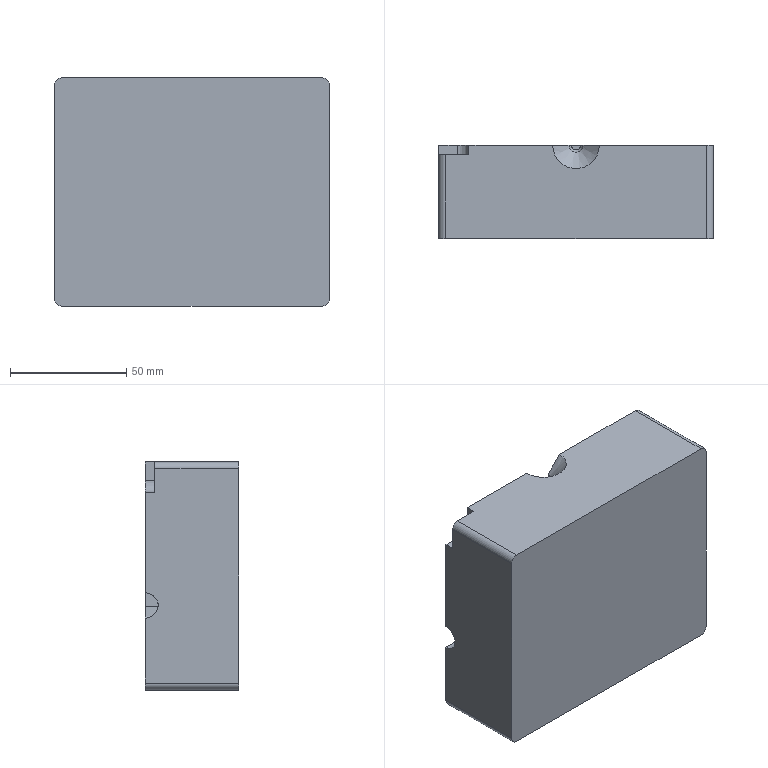NC program | NX | posted with a generic post | part box 118 x 40 x 98 mm
Lines 2681 to 3706 of 39656:
(CONTOUR_AREA , TOOL : B4)
N5348 M6
N5350 G54
N5352 G17 G0 G90 X34.942 Y6.616 S0 M3
N5354 G43 Z30. H0
N5356 Z1.2
N5358 G94 G1 Z-2.023 F250.
N5360 G2 X36.94 Y4.614 R2.
N5362 G1 Y4.41 Z-2.031
N5364 X36.938 Y4.351 Z-2.037
N5366 X36.937 Y4.333 Z-2.04
N5368 X36.906 Y4.326 Z-2.039
N5370 X36.749 Y4.28 Z-2.021
N5372 X36.703 Y4.272 Z-2.019
N5374 X36.7 Y4.271
N5376 X36.569 Y4.211 Z-2.015
N5378 X36.556 Y4.205 Z-2.014
N5380 X36.424 Y4.139 Z-2.012
N5382 X36.353 Y4.099 Z-2.011
N5384 X36.299 Y4.065 Z-2.01
N5386 X36.22 Y4.012 Z-2.009
N5388 X36.181 Y3.984
N5390 X36.069 Y3.896 Z-2.01
N5392 X35.957 Y3.79 Z-2.012
N5394 X35.871 Y3.697 Z-2.009
N5396 X35.8 Y3.611 Z-2.006
N5398 X35.781 Y3.588
N5400 X35.69 Y3.455 Z-2.004
N5402 X35.625 Y3.346 Z-2.003
N5404 X35.558 Y3.211 Z-2.002
N5406 X35.5 Y3.072 Z-2.003
N5408 X35.479 Y3.012 Z-2.004
N5410 X35.451 Y2.921
N5412 X35.435 Y2.861 Z-2.005
N5414 X35.43 Y2.837
N5416 X35.429 Y2.833 Z-1.999
N5418 X35.43 Y2.836 Z-2.004
N5420 X35.422 Y2.802 Z-2.005
N5422 X35.413 Y2.76
N5424 X35.39 Y2.612 Z-2.006
N5426 X35.377 Y2.412 Z-2.007
N5428 Y2.288
N5430 Y1.813 Z-2.009
N5432 Y-1.384 Z-2.01
N5434 Y-2.583 Z-2.008
N5436 Y-3.382 Z-1.999
N5438 Y-3.482 Z-1.998
N5440 Y-3.582 Z-2.
N5442 Y-3.61 Z-2.004
N5444 Y-3.611 Z-2.006
N5446 X35.376 Y-3.613 Z-2.02
N5448 X35.361 Z-2.375
N5450 X35.312 Z-2.767
N5452 X35.304 Z-2.804
N5454 X35.262 Z-3.01
N5456 X35.163 Z-3.365
N5458 X35.095 Z-3.558
N5460 X35.064 Z-3.647
N5462 X35.033 Z-3.717
N5464 X34.965 Z-3.877
N5466 X34.767 Z-4.256
N5468 X34.568 Z-4.565
N5470 X34.37 Z-4.83
N5472 X34.172 Z-5.055
N5474 X33.973 Z-5.255
N5476 X33.775 Z-5.431
N5478 X33.577 Z-5.588
N5480 X33.379 Z-5.728
N5482 X33.18 Z-5.853
N5484 X32.982 Z-5.962
N5486 X32.784 Z-6.062
N5488 X32.585 Z-6.148
N5490 X32.387 Z-6.223
N5492 X32.189 Z-6.287
N5494 X31.991 Z-6.342
N5496 X31.792 Z-6.388
N5498 X31.594 Z-6.423
N5500 X31.396 Z-6.449
N5502 X31.197 Z-6.467
N5504 X30.999 Z-6.475
N5506 X30.801
N5508 X30.603 Z-6.467
N5510 X30.404 Z-6.449
N5512 X30.206 Z-6.423
N5514 X30.008 Z-6.388
N5516 X29.809 Z-6.342
N5518 X29.611 Z-6.287
N5520 X29.413 Z-6.223
N5522 X29.215 Z-6.148
N5524 X29.016 Z-6.061
N5526 X28.818 Z-5.964
N5528 X28.62 Z-5.853
N5530 X28.421 Z-5.728
N5532 X28.223 Z-5.588
N5534 X28.025 Z-5.431
N5536 X27.827 Z-5.255
N5538 X27.628 Z-5.056
N5540 X27.43 Z-4.83
N5542 X27.232 Z-4.565
N5544 X27.033 Z-4.255
N5546 X26.835 Z-3.875
N5548 X26.82 Z-3.842
N5550 X26.736 Z-3.647
N5552 X26.705 Z-3.558
N5554 X26.629 Z-3.343
N5556 X26.587 Z-3.203
N5558 X26.58 Z-3.174
N5560 X26.538 Z-3.01
N5562 X26.533 Z-2.985
N5564 X26.488 Z-2.767
N5566 X26.439 Z-2.375
N5568 X26.437 Y-3.611 Z-2.364
N5570 X26.428 Y-3.582 Z-2.191
N5572 X26.426 Y-3.517 Z-2.156
N5574 Y-3.478 Z-2.137
N5576 X26.425 Y-3.382 Z-2.107
N5578 Y-3.275 Z-2.077
N5580 X26.424 Y-3.182 Z-2.062
N5582 Y-3.02 Z-2.037
N5584 Y-2.983 Z-2.034
N5586 X26.423 Y-2.798 Z-2.021
N5588 Y-2.589 Z-2.014
N5590 Y-2.184 Z-2.01
N5592 Y0.614
N5594 Y2.212 Z-2.007
N5596 Y2.412
N5598 X26.41 Y2.612 Z-2.006
N5600 X26.387 Y2.76 Z-2.005
N5602 X26.376 Y2.812
N5604 X26.365 Y2.861
N5606 X26.349 Y2.921 Z-2.004
N5608 X26.321 Y3.011
N5610 X26.3 Y3.072 Z-2.003
N5612 X26.24 Y3.216
N5614 X26.175 Y3.346 Z-2.005
N5616 X26.101 Y3.471 Z-2.007
N5618 X26.044 Y3.552 Z-2.008
N5620 X26.019 Y3.588 Z-2.009
N5622 X26.001 Y3.61
N5624 X25.929 Y3.697 Z-2.011
N5626 X25.844 Y3.789 Z-2.012
N5628 X25.823 Y3.809 Z-2.013
N5630 X25.731 Y3.897 Z-2.012
N5632 X25.619 Y3.984
N5634 X25.582 Y4.011
N5636 X25.501 Y4.065 Z-2.011
N5638 X25.376 Y4.139 Z-2.01
N5640 X25.237 Y4.208 Z-2.009
N5642 X25.095 Y4.265 Z-2.01
N5644 X25.011 Y4.292 Z-2.008
N5646 X24.894 Y4.326 Z-2.003
N5648 X24.881 Y4.329
N5650 X24.872 Y4.331 Z-2.002
N5652 X24.861 Y4.354
N5654 Y4.394 Z-2.004
N5656 Y5.01 Z-2.007
N5658 Y46.77 Z-2.008
N5660 X24.86 Y48.768 Z-2.005
N5662 X24.861 Y48.968 Z-2.007
N5664 X24.859 Y48.984 Z-2.009
N5666 X24.861 Y48.989 Z-2.096
N5668 X24.868 Y48.999 Z-2.295
N5670 X24.87 Y49. Z-2.364
N5672 X24.872 Z-2.387
N5674 X24.877 Z-2.463
N5676 X24.9 Y48.999 Z-2.698
N5678 X24.906 Z-2.741
N5680 X24.927 Z-2.896
N5682 X24.931 Z-2.92
N5684 X24.952 Z-3.051
N5686 X25.051 Z-3.5
N5688 X25.119 Z-3.741
N5690 X25.15 Z-3.851
N5692 X25.181 Z-3.936
N5694 X25.249 Z-4.128
N5696 X25.447 Z-4.597
N5698 X25.645 Z-4.975
N5700 X25.843 Z-5.302
N5702 X26.042 Z-5.587
N5704 X26.24 Z-5.843
N5706 X26.439 Z-6.07
N5708 X26.636 Z-6.276
N5710 X26.835 Z-6.466
N5712 X27.033 Z-6.639
N5714 X27.232 Z-6.798
N5716 X27.43 Z-6.943
N5718 X27.628 Z-7.076
N5720 X27.827 Z-7.199
N5722 X28.025 Z-7.312
N5724 X28.223 Z-7.414
N5726 X28.421 Z-7.507
N5728 X28.62 Z-7.592
N5730 X28.818 Z-7.669
N5732 X29.016 Z-7.738
N5734 X29.215 Z-7.799
N5736 X29.412 Z-7.852
N5738 X29.611 Z-7.901
N5740 X29.809 Z-7.939
N5742 X30.007 Z-7.973
N5744 X30.205 Z-8.
N5746 X30.404 Z-8.019
N5748 X30.601 Z-8.031
N5750 X30.801 Z-8.038
N5752 X30.999
N5754 X31.197 Z-8.032
N5756 X31.396 Z-8.019
N5758 X31.594 Z-8.
N5760 X31.792 Z-7.973
N5762 X31.99 Z-7.94
N5764 X32.189 Z-7.899
N5766 X32.387 Z-7.853
N5768 X32.585 Z-7.799
N5770 X32.784 Z-7.738
N5772 X32.982 Z-7.669
N5774 X33.18 Z-7.592
N5776 X33.379 Z-7.508
N5778 X33.577 Z-7.414
N5780 X33.775 Z-7.311
N5782 X33.973 Z-7.199
N5784 X34.172 Z-7.076
N5786 X34.37 Z-6.943
N5788 X34.568 Z-6.798
N5790 X34.767 Z-6.64
N5792 X34.964 Z-6.466
N5794 X35.163 Z-6.277
N5796 X35.361 Z-6.07
N5798 X35.56 Z-5.843
N5800 X35.758 Z-5.587
N5802 X35.956 Z-5.303
N5804 X36.154 Z-4.976
N5806 X36.353 Z-4.595
N5808 X36.551 Z-4.128
N5810 X36.567 Z-4.088
N5812 X36.65 Z-3.851
N5814 X36.757 Z-3.473
N5816 X36.799 Z-3.301
N5818 X36.843 Z-3.078
N5820 X36.869 Z-2.919
N5822 X36.873 Z-2.897
N5824 X36.898 Z-2.714
N5826 X36.9 Z-2.698
N5828 X36.921 Y49. Z-2.485
N5830 X36.93 Y48.986 Z-2.363
N5832 X36.935 Y48.971 Z-2.232
N5834 Y48.968 Z-2.219
N5836 X36.936 Y48.941 Z-2.201
N5838 X36.937 Y48.768 Z-2.155
N5840 Y48.679 Z-2.132
N5842 X36.938 Y48.568 Z-2.108
N5844 Y48.432 Z-2.08
N5846 Y48.369 Z-2.07
N5848 X36.939 Y48.202 Z-2.046
N5850 Y48.169 Z-2.043
N5852 Y47.985 Z-2.027
N5854 Y47.776 Z-2.018
N5856 Y47.572 Z-2.013
N5858 Y47.17 Z-2.011
N5860 Y42.374 Z-2.018
N5862 X36.94 Y41.175 Z-2.017
N5864 Y40.182 Z-2.007
N5866 Y39.378 Z-2.002
N5868 Y27.389 Z-2.018
N5870 Y6.811
N5872 Y5.215
N5874 Y4.81 Z-2.019
N5876 Y4.614 Z-2.023
N5878 X36.937 Y4.61 Z-2.123
N5880 Y4.383 Z-2.134
N5882 X36.934 Y4.333 Z-2.141
N5884 X36.913 Y4.327 Z-2.14
N5886 X36.906 Y4.326 Z-2.139
N5888 X36.798 Y4.297 Z-2.127
N5890 X36.749 Y4.281 Z-2.121
N5892 X36.742 Y4.28
N5894 X36.719 Y4.276 Z-2.12
N5896 X36.7 Y4.271 Z-2.119
N5898 X36.645 Y4.246 Z-2.117
N5900 X36.551 Y4.203 Z-2.114
N5902 X36.423 Y4.14 Z-2.112
N5904 X36.353 Y4.1 Z-2.111
N5906 X36.298 Y4.066 Z-2.11
N5908 X36.27 Y4.048
N5910 X36.216 Y4.012 Z-2.109
N5912 X36.189 Y3.992
N5914 X36.062 Y3.892 Z-2.11
N5916 X35.956 Y3.791 Z-2.112
N5918 X35.87 Y3.698 Z-2.109
N5920 X35.798 Y3.611 Z-2.106
N5922 X35.785 Y3.595
N5924 X35.758 Y3.559 Z-2.105
N5926 X35.698 Y3.471 Z-2.104
N5928 X35.661 Y3.411
N5930 X35.624 Y3.347 Z-2.103
N5932 X35.56 Y3.22 Z-2.102
N5934 X35.544 Y3.186
N5936 X35.493 Y3.058 Z-2.103
N5938 X35.476 Y3.012 Z-2.104
N5940 X35.463 Y2.966
N5942 X35.45 Y2.923
N5944 X35.428 Y2.84 Z-2.105
N5946 X35.421 Y2.812
N5948 X35.414 Y2.773
N5950 X35.411 Y2.761
N5952 X35.388 Y2.612 Z-2.106
N5954 X35.375 Y2.414 Z-2.107
N5956 Y0.182 Z-2.109
N5958 Y-1.384 Z-2.11
N5960 Y-2.448 Z-2.108
N5962 Y-3.505 Z-2.099
N5964 Y-3.507 Z-2.101
N5966 Y-3.51 Z-2.103
N5968 X35.374 Y-3.511 Z-2.156
N5970 X35.366 Y-3.513 Z-2.299
N5972 X35.361 Z-2.375
N5974 X35.312 Z-2.761
N5976 X35.262 Z-3.006
N5978 X35.213 Z-3.199
N5980 X35.163 Z-3.365
N5982 X35.064 Z-3.644
N5984 X34.965 Z-3.877
N5986 X34.767 Z-4.256
N5988 X34.568 Z-4.565
N5990 X34.37 Z-4.83
N5992 X34.172 Z-5.055
N5994 X33.973 Z-5.255
N5996 X33.775 Z-5.431
N5998 X33.577 Z-5.588
N6000 X33.379 Z-5.728
N6002 X33.18 Z-5.853
N6004 X32.982 Z-5.962
N6006 X32.784 Z-6.062
N6008 X32.585 Z-6.148
N6010 X32.387 Z-6.223
N6012 X32.189 Z-6.287
N6014 X31.991 Z-6.342
N6016 X31.792 Z-6.388
N6018 X31.594 Z-6.423
N6020 X31.396 Z-6.449
N6022 X31.197 Z-6.467
N6024 X30.999 Z-6.475
N6026 X30.801
N6028 X30.603 Z-6.467
N6030 X30.404 Z-6.449
N6032 X30.206 Z-6.423
N6034 X30.008 Z-6.388
N6036 X29.809 Z-6.342
N6038 X29.611 Z-6.287
N6040 X29.413 Z-6.223
N6042 X29.215 Z-6.148
N6044 X29.016 Z-6.061
N6046 X28.818 Z-5.964
N6048 X28.62 Z-5.853
N6050 X28.421 Z-5.728
N6052 X28.223 Z-5.588
N6054 X28.025 Z-5.431
N6056 X27.827 Z-5.255
N6058 X27.628 Z-5.056
N6060 X27.43 Z-4.83
N6062 X27.232 Z-4.565
N6064 X27.033 Z-4.255
N6066 X26.835 Z-3.875
N6068 X26.736 Z-3.644
N6070 X26.637 Z-3.365
N6072 X26.587 Z-3.199
N6074 X26.538 Z-3.006
N6076 X26.505 Z-2.846
N6078 X26.488 Z-2.761
N6080 X26.456 Y-3.511 Z-2.512
N6082 X26.439 Y-3.502 Z-2.375
N6084 X26.433 Y-3.488 Z-2.277
N6086 X26.432 Y-3.484 Z-2.263
N6088 X26.43 Y-3.382 Z-2.215
N6090 X26.429 Y-3.342 Z-2.2
N6092 X26.426 Y-3.182 Z-2.16
N6094 Y-3.161 Z-2.156
N6096 Y-2.949 Z-2.131
N6098 Y-2.787 Z-2.12
N6100 X26.425 Y-2.732 Z-2.118
N6102 Y-2.585 Z-2.114
N6104 Y-2.184 Z-2.11
N6106 Y0.614
N6108 Y2.212 Z-2.107
N6110 Y2.412
N6112 X26.418 Y2.513 Z-2.106
N6114 X26.412 Y2.612
N6116 X26.389 Y2.761 Z-2.105
N6118 X26.386 Y2.773
N6120 X26.379 Y2.812
N6122 X26.372 Y2.84
N6124 X26.35 Y2.923 Z-2.104
N6126 X26.338 Y2.964
N6128 X26.324 Y3.012
N6130 X26.307 Y3.058 Z-2.103
N6132 X26.297 Y3.087
N6134 X26.258 Y3.181
N6136 X26.245 Y3.211 Z-2.102
N6138 X26.24 Y3.22 Z-2.103
N6140 X26.176 Y3.347 Z-2.105
N6142 X26.139 Y3.411 Z-2.106
N6144 X26.102 Y3.471 Z-2.107
N6146 X26.043 Y3.557 Z-2.108
N6148 X26.02 Y3.588 Z-2.109
N6150 X26.003 Y3.61
N6152 X25.93 Y3.698 Z-2.111
N6154 X25.834 Y3.801 Z-2.113
N6156 X25.731 Y3.897 Z-2.112
N6158 X25.61 Y3.992
N6160 X25.502 Y4.066 Z-2.111
N6162 X25.472 Y4.085
N6164 X25.447 Y4.1 Z-2.11
N6166 X25.387 Y4.134
N6168 X25.377 Y4.14
N6170 X25.249 Y4.203 Z-2.109
N6172 X25.233 Y4.211
N6174 X25.095 Y4.265 Z-2.11
N6176 X25.082 Y4.27
N6178 X24.969 Y4.306 Z-2.107
N6180 X24.872 Y4.331 Z-2.102
N6182 X24.864 Y4.349
N6184 X24.862 Y4.497 Z-2.104
N6186 Y4.899 Z-2.106
N6188 Y5.099 Z-2.107
N6190 Y46.77 Z-2.108
N6192 Y48.568 Z-2.105
N6194 Y48.656 Z-2.106
N6196 Y48.768 Z-2.107
N6198 Y48.861 Z-2.111
N6200 X24.863 Y48.88 Z-2.116
N6202 Y48.887 Z-2.141
N6204 X24.865 Y48.895 Z-2.231
N6206 X24.873 Y48.899 Z-2.393
N6208 X24.877 Y48.9 Z-2.453
N6210 X24.902 Y48.899 Z-2.706
N6212 X24.927 Z-2.889
N6214 X24.952 Z-3.045
N6216 X25.001 Z-3.291
N6218 X25.051 Z-3.5
N6220 X25.15 Z-3.847
N6222 X25.249 Z-4.128
N6224 X25.447 Z-4.597
N6226 X25.646 Z-4.976
N6228 X25.844 Z-5.303
N6230 X26.042 Z-5.587
N6232 X26.24 Z-5.843
N6234 X26.439 Z-6.07
N6236 X26.637 Z-6.277
N6238 X26.835 Z-6.467
N6240 X27.033 Z-6.639
N6242 X27.232 Z-6.798
N6244 X27.43 Z-6.943
N6246 X27.628 Z-7.076
N6248 X27.827 Z-7.199
N6250 X28.025 Z-7.312
N6252 X28.223 Z-7.414
N6254 X28.421 Z-7.507
N6256 X28.62 Z-7.592
N6258 X28.818 Z-7.669
N6260 X29.016 Z-7.738
N6262 X29.215 Z-7.799
N6264 X29.413 Z-7.853
N6266 X29.611 Z-7.901
N6268 X29.809 Z-7.939
N6270 X30.008 Z-7.973
N6272 X30.206 Z-8.
N6274 X30.404 Z-8.019
N6276 X30.603 Z-8.031
N6278 X30.801 Z-8.038
N6280 X30.999
N6282 X31.197 Z-8.032
N6284 X31.396 Z-8.019
N6286 X31.594 Z-8.
N6288 X31.792 Z-7.973
N6290 X31.991 Z-7.94
N6292 X32.189 Z-7.899
N6294 X32.387 Z-7.853
N6296 X32.585 Z-7.799
N6298 X32.784 Z-7.738
N6300 X32.982 Z-7.669
N6302 X33.18 Z-7.592
N6304 X33.379 Z-7.508
N6306 X33.577 Z-7.414
N6308 X33.775 Z-7.311
N6310 X33.973 Z-7.199
N6312 X34.172 Z-7.076
N6314 X34.37 Z-6.943
N6316 X34.568 Z-6.798
N6318 X34.767 Z-6.64
N6320 X34.965 Z-6.466
N6322 X35.163 Z-6.277
N6324 X35.361 Z-6.07
N6326 X35.56 Z-5.843
N6328 X35.758 Z-5.587
N6330 X35.956 Z-5.303
N6332 X36.154 Z-4.976
N6334 X36.353 Z-4.595
N6336 X36.551 Z-4.128
N6338 X36.65 Z-3.847
N6340 X36.749 Z-3.5
N6342 X36.799 Z-3.295
N6344 X36.827 Z-3.152
N6346 X36.844 Z-3.064
N6348 X36.873 Z-2.889
N6350 X36.882 Z-2.826
N6352 X36.898 Z-2.706
N6354 X36.907 Y48.898 Z-2.617
N6356 X36.923 Y48.892 Z-2.453
N6358 X36.925 Y48.89 Z-2.417
N6360 X36.929 Y48.883 Z-2.362
N6362 X36.932 Y48.871 Z-2.298
N6364 Y48.862 Z-2.292
N6366 X36.933 Y48.838 Z-2.277
N6368 X36.936 Y48.589 Z-2.213
N6370 Y48.392 Z-2.175
N6372 X36.937 Y48.184 Z-2.145
N6374 Y47.969 Z-2.127
N6376 Y47.87 Z-2.122
N6378 Y47.773 Z-2.118
N6380 X36.938 Y47.571 Z-2.113
N6382 Y47.17 Z-2.111
N6384 Y41.975 Z-2.117
N6386 Y41.265 Z-2.116
N6388 Y41.064 Z-2.115
N6390 Y40.18 Z-2.107
N6392 Y39.378 Z-2.102
N6394 Y27.389 Z-2.118
N6396 Y4.908 Z-2.119
N6398 Y4.711 Z-2.121
N6400 X36.937 Y4.61 Z-2.123
N6402 X36.935 Z-2.222
N6404 Z-2.224
N6406 Y4.402 Z-2.233
N6408 X36.933 Y4.333 Z-2.241
N6410 X36.884 Y4.321 Z-2.237
N6412 X36.868 Y4.316 Z-2.236
N6414 X36.829 Y4.308 Z-2.231
N6416 X36.804 Y4.3 Z-2.228
N6418 X36.749 Y4.282 Z-2.222
N6420 X36.7 Y4.271 Z-2.219
N6422 X36.553 Y4.205 Z-2.214
N6424 X36.422 Y4.141 Z-2.212
N6426 X36.353 Y4.101 Z-2.211
N6428 X36.297 Y4.067 Z-2.21
N6430 X36.279 Y4.055
N6432 X36.213 Y4.011 Z-2.209
N6434 X36.201 Y4.003
N6436 X36.056 Y3.888 Z-2.211
N6438 X35.956 Y3.794 Z-2.212
N6440 X35.933 Y3.769 Z-2.211
N6442 X35.888 Y3.729 Z-2.21
N6444 X35.863 Y3.705 Z-2.209
N6446 X35.834 Y3.665 Z-2.208
N6448 X35.816 Y3.636 Z-2.207
N6450 X35.76 Y3.563 Z-2.205
N6452 X35.743 Y3.539
N6454 X35.697 Y3.473 Z-2.204
N6456 X35.622 Y3.348 Z-2.203
N6458 X35.553 Y3.212 Z-2.202
N6460 X35.53 Y3.161 Z-2.203
N6462 X35.496 Y3.076
N6464 X35.484 Y3.039
N6466 X35.474 Y3.012 Z-2.204
N6468 X35.444 Y2.909
N6470 X35.406 Y2.766 Z-2.205
N6472 X35.4 Y2.719
N6474 X35.386 Y2.612 Z-2.206
N6476 X35.374 Y2.447 Z-2.207
N6478 X35.371 Y2.412
N6480 Y2.212
N6482 Y1.765 Z-2.209
N6484 Y-1.384 Z-2.21
N6486 Y-2.431 Z-2.208
N6488 Y-2.63 Z-2.207
N6490 Y-3.225 Z-2.202
N6492 Y-3.382 Z-2.209
N6494 X35.362 Y-3.409 Z-2.358
N6496 X35.361 Y-3.41 Z-2.375
N6498 X35.323 Y-3.413 Z-2.67
N6500 X35.312 Z-2.761
N6502 X35.262 Z-3.006
N6504 X35.213 Z-3.199
N6506 X35.163 Z-3.365
N6508 X35.064 Z-3.644
N6510 X34.965 Z-3.877
N6512 X34.767 Z-4.256
N6514 X34.568 Z-4.565
N6516 X34.37 Z-4.83
N6518 X34.172 Z-5.055
N6520 X33.973 Z-5.255
N6522 X33.775 Z-5.431
N6524 X33.577 Z-5.588
N6526 X33.379 Z-5.728
N6528 X33.18 Z-5.853
N6530 X32.982 Z-5.962
N6532 X32.784 Z-6.062
N6534 X32.585 Z-6.148
N6536 X32.387 Z-6.223
N6538 X32.189 Z-6.287
N6540 X31.991 Z-6.342
N6542 X31.792 Z-6.388
N6544 X31.594 Z-6.423
N6546 X31.396 Z-6.449
N6548 X31.197 Z-6.467
N6550 X30.999 Z-6.475
N6552 X30.801
N6554 X30.603 Z-6.467
N6556 X30.404 Z-6.449
N6558 X30.206 Z-6.423
N6560 X30.008 Z-6.388
N6562 X29.809 Z-6.342
N6564 X29.611 Z-6.287
N6566 X29.413 Z-6.223
N6568 X29.215 Z-6.148
N6570 X29.016 Z-6.061
N6572 X28.818 Z-5.964
N6574 X28.62 Z-5.853
N6576 X28.421 Z-5.728
N6578 X28.223 Z-5.588
N6580 X28.025 Z-5.431
N6582 X27.827 Z-5.255
N6584 X27.628 Z-5.056
N6586 X27.43 Z-4.83
N6588 X27.232 Z-4.565
N6590 X27.033 Z-4.255
N6592 X26.835 Z-3.875
N6594 X26.736 Z-3.644
N6596 X26.637 Z-3.365
N6598 X26.587 Z-3.199
N6600 X26.538 Z-3.006
N6602 X26.488 Z-2.761
N6604 X26.439 Y-3.408 Z-2.375
N6606 X26.437 Y-3.406 Z-2.353
N6608 Y-3.405 Z-2.35
N6610 X26.436 Y-3.393 Z-2.332
N6612 Y-3.382 Z-2.324
N6614 X26.434 Y-3.289 Z-2.288
N6616 X26.433 Y-3.268 Z-2.282
N6618 X26.432 Y-3.182 Z-2.264
N6620 Y-3.1 Z-2.249
N6622 X26.431 Y-2.983 Z-2.237
N6624 X26.43 Y-2.915 Z-2.23
N6626 Y-2.783 Z-2.222
N6628 Y-2.725 Z-2.219
N6630 Y-2.583 Z-2.215
N6632 Y-2.53 Z-2.214
N6634 X26.429 Y-1.984 Z-2.21
N6636 Y0.614
N6638 Y2.247 Z-2.207
N6640 Y2.412
N6642 X26.426 Y2.447
N6644 X26.414 Y2.612 Z-2.206
N6646 X26.4 Y2.719 Z-2.205
N6648 X26.394 Y2.766
N6650 X26.382 Y2.812
N6652 X26.348 Y2.938 Z-2.204
N6654 X26.326 Y3.012
N6656 X26.287 Y3.119 Z-2.203
N6658 X26.24 Y3.226
N6660 X26.215 Y3.278
N6662 X26.178 Y3.348 Z-2.205
N6664 X26.135 Y3.422 Z-2.206
N6666 X26.103 Y3.473 Z-2.207
N6668 X26.012 Y3.601 Z-2.209
N6670 X25.934 Y3.702 Z-2.21
N6672 X25.882 Y3.753 Z-2.212
N6674 X25.826 Y3.811 Z-2.213
N6676 X25.764 Y3.869 Z-2.212
N6678 X25.732 Y3.898
N6680 X25.602 Y4.
N6682 X25.447 Y4.102 Z-2.21
N6684 X25.416 Y4.12
N6686 X25.378 Y4.141
N6688 X25.249 Y4.204 Z-2.209
N6690 X25.235 Y4.211
N6692 X25.074 Y4.273 Z-2.21
N6694 X24.97 Y4.307 Z-2.207
N6696 X24.945 Y4.313 Z-2.206
N6698 X24.932 Y4.316 Z-2.205
N6700 X24.929 Y4.322
N6702 X24.921 Y4.319
N6704 X24.872 Y4.331 Z-2.203
N6706 X24.867 Y4.343 Z-2.202
N6708 X24.864 Y4.41 Z-2.204
N6710 Y4.973 Z-2.207
N6712 Y5.173
N6714 Y46.734 Z-2.208
N6716 Y48.746 Z-2.206
N6718 Y48.768 Z-2.208
N6720 Y48.789 Z-2.212
N6722 Y48.791 Z-2.214
N6724 X24.865 Y48.794 Z-2.231
N6726 X24.871 Y48.799 Z-2.362
N6728 X24.877 Y48.8 Z-2.453
N6730 X24.902 Y48.799 Z-2.706
N6732 X24.927 Z-2.889
N6734 X24.952 Z-3.045
N6736 X25.001 Z-3.291
N6738 X25.051 Z-3.5
N6740 X25.15 Z-3.847
N6742 X25.249 Z-4.128
N6744 X25.447 Z-4.597
N6746 X25.646 Z-4.976
N6748 X25.844 Z-5.303
N6750 X26.042 Z-5.587
N6752 X26.24 Z-5.843
N6754 X26.439 Z-6.07
N6756 X26.637 Z-6.277
N6758 X26.835 Z-6.467
N6760 X27.033 Z-6.639
N6762 X27.232 Z-6.798
N6764 X27.43 Z-6.943
N6766 X27.628 Z-7.076
N6768 X27.827 Z-7.199
N6770 X28.025 Z-7.312
N6772 X28.223 Z-7.414
N6774 X28.421 Z-7.507
N6776 X28.62 Z-7.592
N6778 X28.818 Z-7.669
N6780 X29.016 Z-7.738
N6782 X29.215 Z-7.799
N6784 X29.413 Z-7.853
N6786 X29.611 Z-7.901
N6788 X29.809 Z-7.939
N6790 X30.008 Z-7.973
N6792 X30.206 Z-8.
N6794 X30.404 Z-8.019
N6796 X30.603 Z-8.031
N6798 X30.801 Z-8.038
N6800 X30.999
N6802 X31.197 Z-8.032
N6804 X31.396 Z-8.019
N6806 X31.594 Z-8.
N6808 X31.792 Z-7.973
N6810 X31.991 Z-7.94
N6812 X32.189 Z-7.899
N6814 X32.387 Z-7.853
N6816 X32.585 Z-7.799
N6818 X32.784 Z-7.738
N6820 X32.982 Z-7.669
N6822 X33.18 Z-7.592
N6824 X33.379 Z-7.508
N6826 X33.577 Z-7.414
N6828 X33.775 Z-7.311
N6830 X33.973 Z-7.199
N6832 X34.172 Z-7.076
N6834 X34.37 Z-6.943
N6836 X34.568 Z-6.798
N6838 X34.767 Z-6.64
N6840 X34.965 Z-6.466
N6842 X35.163 Z-6.277
N6844 X35.361 Z-6.07
N6846 X35.56 Z-5.843
N6848 X35.758 Z-5.587
N6850 X35.956 Z-5.303
N6852 X36.154 Z-4.976
N6854 X36.353 Z-4.595
N6856 X36.551 Z-4.128
N6858 X36.65 Z-3.847
N6860 X36.749 Z-3.5
N6862 X36.799 Z-3.295
N6864 X36.847 Z-3.045
N6866 X36.873 Z-2.889
N6868 X36.892 Z-2.749
N6870 X36.898 Z-2.706
N6872 X36.917 Y48.796 Z-2.508
N6874 X36.919 Z-2.488
N6876 X36.929 Y48.782 Z-2.368
N6878 Y48.765 Z-2.36
N6880 X36.931 Y48.568 Z-2.314
N6882 X36.933 Y48.456 Z-2.288
N6884 X36.935 Y48.169 Z-2.245
N6886 Y48.035 Z-2.232
N6888 Y47.969 Z-2.227
N6890 Y47.77 Z-2.218
N6892 X36.936 Y47.57 Z-2.213
N6894 Y47.17 Z-2.211
N6896 Y42.389 Z-2.217
N6898 Y41.175 Z-2.216
N6900 Y40.197 Z-2.207
N6902 Y39.377 Z-2.202
N6904 X36.935 Y27.399 Z-2.218
N6906 Y5.214
N6908 Y4.813 Z-2.219
N6910 Y4.672 Z-2.222
N6912 Y4.61 Z-2.224
N6914 X36.931 Z-2.323
N6916 X36.93 Y4.41 Z-2.332
N6918 Y4.363 Z-2.339
N6920 Y4.343 Z-2.34
N6922 Y4.333 Z-2.341
N6924 X36.888 Y4.323 Z-2.339
N6926 X36.829 Y4.308 Z-2.332
N6928 X36.764 Y4.287 Z-2.324
N6930 X36.749 Y4.283 Z-2.322
N6932 X36.714 Y4.277 Z-2.32
N6934 X36.551 Y4.207 Z-2.314
N6936 X36.504 Y4.184
N6938 X36.421 Y4.142 Z-2.312
N6940 X36.317 Y4.082 Z-2.31
N6942 X36.176 Y3.989 Z-2.309
N6944 X36.058 Y3.894 Z-2.31
N6946 X35.956 Y3.799 Z-2.312
N6948 X35.937 Y3.779 Z-2.311
N6950 X35.917 Y3.757
N6952 X35.863 Y3.705 Z-2.309
N6954 X35.831 Y3.66 Z-2.308
N6956 X35.79 Y3.611 Z-2.306
N6958 X35.758 Y3.57 Z-2.305
N6960 X35.651 Y3.411 Z-2.303
N6962 X35.591 Y3.3
N6964 X35.547 Y3.212 Z-2.302
N6966 X35.487 Y3.065 Z-2.303
N6968 X35.468 Y3.012
N6970 X35.46 Y2.986 Z-2.304
N6972 X35.449 Y2.95
N6974 X35.443 Y2.929
N6976 X35.411 Y2.804 Z-2.305
N6978 X35.4 Y2.773
N6980 X35.389 Y2.683
N6982 X35.379 Y2.612 Z-2.306
N6984 X35.365 Y2.397 Z-2.307
N6986 Y0.244 Z-2.309
N6988 Y-1.324 Z-2.31
N6990 Y-2.522 Z-2.308
N6992 X35.366 Y-3.296 Z-2.301
N6994 X35.365 Y-3.298 Z-2.306
N6996 X35.361 Y-3.305 Z-2.375
N6998 X35.344 Y-3.312 Z-2.51
N7000 X35.312 Y-3.313 Z-2.761
N7002 X35.295 Z-2.846
N7004 X35.262 Z-3.006
N7006 X35.213 Z-3.199
N7008 X35.163 Z-3.365
N7010 X35.064 Z-3.644
N7012 X34.965 Z-3.877
N7014 X34.767 Z-4.256
N7016 X34.568 Z-4.565
N7018 X34.37 Z-4.83
N7020 X34.172 Z-5.055
N7022 X33.973 Z-5.255
N7024 X33.775 Z-5.431
N7026 X33.577 Z-5.588
N7028 X33.379 Z-5.728
N7030 X33.18 Z-5.853
N7032 X32.982 Z-5.963
N7034 X32.784 Z-6.062
N7036 X32.585 Z-6.148
N7038 X32.387 Z-6.223
N7040 X32.189 Z-6.287
N7042 X31.991 Z-6.342
N7044 X31.792 Z-6.388
N7046 X31.594 Z-6.423
N7048 X31.396 Z-6.449
N7050 X31.197 Z-6.467
N7052 X30.999 Z-6.475
N7054 X30.801
N7056 X30.603 Z-6.467
N7058 X30.404 Z-6.449
N7060 X30.206 Z-6.423
N7062 X30.008 Z-6.388
N7064 X29.809 Z-6.342
N7066 X29.611 Z-6.287
N7068 X29.413 Z-6.223
N7070 X29.215 Z-6.148
N7072 X29.016 Z-6.061
N7074 X28.818 Z-5.964
N7076 X28.62 Z-5.853
N7078 X28.421 Z-5.728
N7080 X28.223 Z-5.588
N7082 X28.025 Z-5.431
N7084 X27.827 Z-5.255
N7086 X27.628 Z-5.056
N7088 X27.43 Z-4.83
N7090 X27.232 Z-4.565
N7092 X27.033 Z-4.255
N7094 X26.835 Z-3.875
N7096 X26.736 Z-3.644
N7098 X26.637 Z-3.365
N7100 X26.587 Z-3.199
N7102 X26.538 Z-3.006
N7104 X26.488 Z-2.761
N7106 X26.456 Y-3.312 Z-2.511
N7108 X26.447 Y-3.307 Z-2.444
N7110 X26.444 Y-3.303 Z-2.416
N7112 X26.439 Y-3.232 Z-2.375
N7114 X26.438 Y-3.182 Z-2.364
N7116 X26.437 Y-3.041 Z-2.343
N7118 Y-3.015 Z-2.339
N7120 X26.436 Y-2.83 Z-2.323
N7122 X26.435 Y-2.583 Z-2.314
N7124 Y-2.063 Z-2.31
N7126 Y0.554
N7128 Y2.301 Z-2.307
N7130 X26.434 Y2.412
N7132 X26.426 Y2.536 Z-2.306
N7134 X26.421 Y2.612
N7136 X26.414 Y2.661 Z-2.305
N7138 X26.4 Y2.773
N7140 X26.389 Y2.804
N7142 X26.387 Y2.812
N7144 X26.351 Y2.95 Z-2.304
N7146 X26.34 Y2.986
N7148 X26.332 Y3.012 Z-2.303
N7150 X26.291 Y3.122
N7152 X26.249 Y3.22 Z-2.302
N7154 X26.175 Y3.365 Z-2.305
N7156 X26.149 Y3.411
N7158 X26.042 Y3.57 Z-2.308
N7160 X26.01 Y3.611 Z-2.309
N7162 X25.968 Y3.662 Z-2.31
N7164 X25.937 Y3.705 Z-2.311
N7166 X25.884 Y3.757 Z-2.312
N7168 X25.863 Y3.779
N7170 X25.799 Y3.842
N7172 X25.767 Y3.871
N7174 X25.734 Y3.9
N7176 X25.621 Y3.992
N7178 X25.505 Y4.069 Z-2.311
N7180 X25.447 Y4.104 Z-2.31
N7182 X25.444 Y4.106
N7184 X25.379 Y4.142
N7186 X25.239 Y4.211 Z-2.309
N7188 X25.097 Y4.267 Z-2.31
N7190 X25.071 Y4.276
N7192 X25.051 Y4.283
N7194 X24.971 Y4.307 Z-2.307
N7196 X24.933 Y4.317 Z-2.305
N7198 X24.932 Y4.318
N7200 X24.929 Y4.324
N7202 X24.894 Y4.326 Z-2.304
N7204 X24.879 Y4.33 Z-2.303
N7206 X24.873 Y4.332
N7208 X24.871 Y4.338 Z-2.302
N7210 X24.869 Y4.41 Z-2.304
N7212 Y4.94 Z-2.307
N7214 Y5.139
N7216 X24.868 Y46.77 Z-2.308
N7218 Y48.454 Z-2.306
N7220 Y48.568 Z-2.307
N7222 X24.869 Y48.645 Z-2.312
N7224 Y48.689 Z-2.327
N7226 X24.871 Y48.696 Z-2.362
N7228 X24.873 Y48.699 Z-2.394
N7230 X24.877 Y48.7 Z-2.453
N7232 X24.886 Z-2.54
N7234 X24.902 Y48.699 Z-2.706
N7236 X24.927 Z-2.889
N7238 X24.952 Z-3.045
N7240 X25.001 Z-3.291
N7242 X25.051 Z-3.5
N7244 X25.15 Z-3.847
N7246 X25.249 Z-4.128
N7248 X25.447 Z-4.597
N7250 X25.646 Z-4.976
N7252 X25.844 Z-5.303
N7254 X26.042 Z-5.587
N7256 X26.24 Z-5.843
N7258 X26.439 Z-6.07
N7260 X26.637 Z-6.277
N7262 X26.835 Z-6.467
N7264 X27.033 Z-6.639
N7266 X27.232 Z-6.798
N7268 X27.43 Z-6.943
N7270 X27.628 Z-7.076
N7272 X27.827 Z-7.199
N7274 X28.025 Z-7.312
N7276 X28.223 Z-7.414
N7278 X28.421 Z-7.507
N7280 X28.62 Z-7.592
N7282 X28.818 Z-7.669
N7284 X29.016 Z-7.738
N7286 X29.215 Z-7.799
N7288 X29.413 Z-7.853
N7290 X29.611 Z-7.901
N7292 X29.809 Z-7.94
N7294 X30.008 Z-7.973
N7296 X30.206 Z-8.
N7298 X30.404 Z-8.019
N7300 X30.603 Z-8.031
N7302 X30.801 Z-8.038
N7304 X30.999
N7306 X31.197 Z-8.032
N7308 X31.396 Z-8.019
N7310 X31.594 Z-8.
N7312 X31.792 Z-7.973
N7314 X31.991 Z-7.94
N7316 X32.189 Z-7.899
N7318 X32.387 Z-7.853
N7320 X32.585 Z-7.799
N7322 X32.784 Z-7.738
N7324 X32.982 Z-7.669
N7326 X33.18 Z-7.592
N7328 X33.379 Z-7.508
N7330 X33.577 Z-7.414
N7332 X33.775 Z-7.311
N7334 X33.973 Z-7.199
N7336 X34.172 Z-7.076
N7338 X34.37 Z-6.943
N7340 X34.568 Z-6.798
N7342 X34.767 Z-6.64
N7344 X34.965 Z-6.466
N7346 X35.163 Z-6.277
N7348 X35.361 Z-6.07
N7350 X35.56 Z-5.843
N7352 X35.758 Z-5.587
N7354 X35.956 Z-5.303
N7356 X36.154 Z-4.976
N7358 X36.353 Z-4.595
N7360 X36.551 Z-4.128
N7362 X36.65 Z-3.847
N7364 X36.749 Z-3.5
N7366 X36.799 Z-3.295
N7368 X36.848 Z-3.039
N7370 X36.873 Z-2.889
N7372 X36.882 Z-2.826
N7374 X36.898 Y48.698 Z-2.706
N7376 X36.907 Y48.696 Z-2.615
N7378 X36.923 Y48.684 Z-2.453
N7380 X36.925 Y48.568 Z-2.421
N7382 X36.928 Y48.41 Z-2.381
N7384 Y48.369 Z-2.374
N7386 X36.929 Y48.295 Z-2.362
N7388 X36.93 Y48.172 Z-2.345
N7390 Y48.137 Z-2.341
N7392 X36.931 Y47.969 Z-2.328